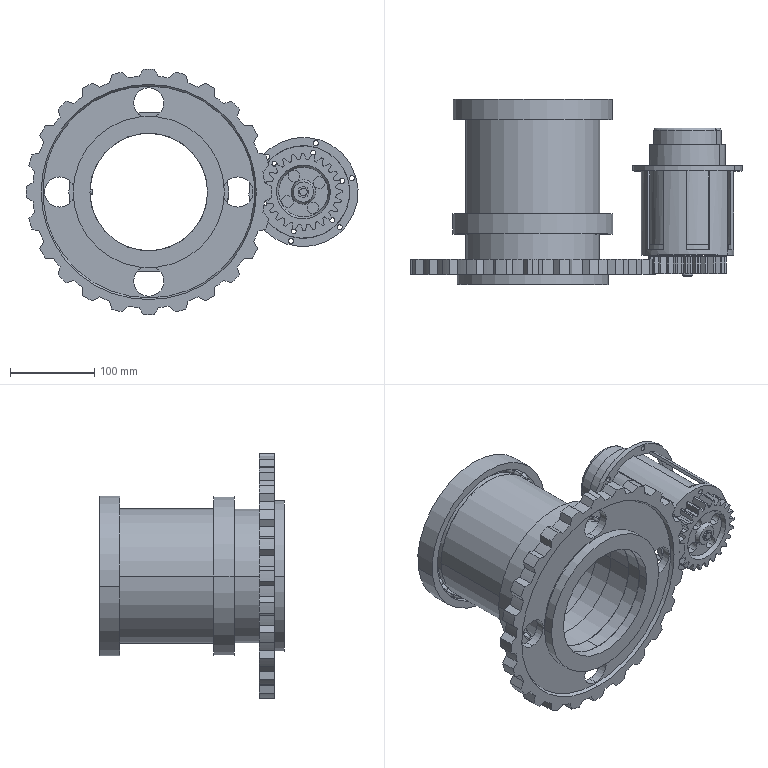Part | NX | features BREP 44 | 80 solids | 675 faces | box 395 x 220 x 292 mm | volume 2964595 mm3 | sphere 264 | cylinder 209 | plane 168 | cone 20 | torus 14 | commonest cylinder face diameters 92 x25 292 x25 78 x24 276 x24 6 x14 140 x13